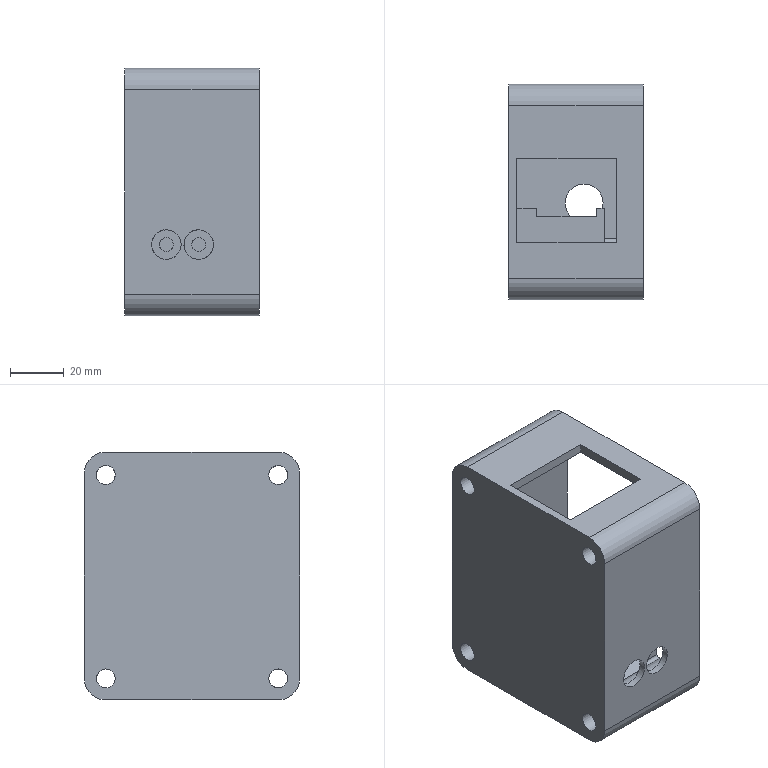NC program | NX | posted by the shop | part box 50 x 80 x 92 mm
Lines 1 to 169 of 30419:
%
O1234(1)
(T=1 D63 face mill Z=-30.00 D=63.00 R=0.00 L=30.00)
()
(T=3 Drill D7.0-73-105 Z=-73.00 D=7.00 R=0.00 L=105.00)
(T=4 Drill D4.0-54-83 Z=-54.00 D=4.00 R=0.00 L=83.00)
(T=5 D4-12-D4-50-3T-rough Z=-12.00 D=4.00 R=0.00 L=50.00)
(T=6 D12-36-D12-120-3T-finish Z=-45.00 D=12.00 R=0.00 L=120.00)
(T=7 D6-18-D6-50-3T-rough Z=-18.00 D=6.00 R=0.00 L=50.00)
(T=9 D2-6-D4-50-3T-rough Z=-6.00 D=2.00 R=0.00 L=7.00)
(T=10 D10-1 Z=-4.00 D=16.00 R=0.00 L=50.00)
()
(T=13 Drill D2.5-35-61 Z=-36.00 D=2.50 R=0.00 L=61.00)
(T=14 Spiral flute tap M3-10-D4-52 Z=-10.00 D=3.00 R=0.00 L=12.00)
G40 G17 G80 G90 G21
M9
M5
G91 G28 Z0.0
M1
N1
(T=1 N=D63 face mill D=1.00 R=0.00 FL=10.00 L=11.00)
(XY-STOCK=0.05)
T1 M6
T2
G0 G90 G54 X-22.5 Y-113. S4000 M3
G43 H01 Z30.
M8
Z3.
G1 Z0.0 F1000.
Y-50.
Y50.
Y113.
Z3.
G0 Z30.
X32.5 Y-113.
Z3.
G1 Z0.0
Y-50.
Y50.
Y113.
Z3.
G0 Z30.
M9
M5
G91 G28 Z0.0
M1
N2
(T=2 N=点孔D8-120-90度 D=8.00 R=0.00 FL=0.00 L=120.00)
(XY-STOCK=0.00)
T2 M6
T3
G0 G90 G54 X-40.5 Y17. S3000 M3
G43 H02 Z30.
M8
G98 G81 X-40.5 Y17. Z-1.5 R3. F200.
X-35.917 Y20.
X-29.422 Y27.
X-28.668 Y35.5
X-5.083 Y20.
X4.083
X29.168 Y35.5
X29.922 Y27.
X34.917 Y20.
X39.5 Y17.
Y-17.
X34.764 Y-20.027
X29.168 Y-35.5
X4.083 Y-20.
X-5.083
X-28.668 Y-35.5
X-29.422 Y-27.
X-35.917 Y-20.
G80
G0 X-35.917 Y-20. Z30.
G0 X-37.5 Y-32. S3000 M3
M8
G98 G81 X-37.5 Y-32. Z-1.5 R3. F200.
Y32.
X38.
Y-32.
G80
G0 X38. Y-32. Z30.
M9
M5
G91 G28 Z0.0
M1
N3
(T=3 N=Drill D7.0-73-105 D=7.00 R=0.00 FL=73.00 L=105.00)
(XY-STOCK=0.00)
T3 M6
T4
G0 G90 G54 X-37.5 Y-32. S3000 M3
G43 H03 Z30.
M8
G98 G83 X-37.5 Y-32. Z-54. R3. F250. Q2.
Y32.
X38.
Y-32.
G80
G0 X38. Y-32. Z30.
M9
M5
G91 G28 Z0.0
M1
N4
(T=4 N=Drill D4.0-54-83 D=4.00 R=0.00 FL=54.00 L=83.00)
(XY-STOCK=0.00)
T4 M6
T5
G0 G90 G54 X-40.5 Y17. S3000 M3
G43 H04 Z30.
M8
G98 G83 X-40.5 Y17. Z-47. R3. F200. Q2.
X-35.917 Y20.
X-29.422 Y27.
X-28.668 Y35.5
X-5.083 Y20.
X4.083
X29.168 Y35.5
X29.922 Y27.
X34.917 Y20.
X39.5 Y17.
Y-17.
X34.764 Y-20.027
X29.168 Y-35.5
X4.083 Y-20.
X-5.083
X-28.668 Y-35.5
X-29.422 Y-27.
X-35.917 Y-20.
G80
G0 X-35.917 Y-20. Z30.
M9
M5
G91 G28 Z0.0
M1
N5
(T=5 N=D4-12-D4-50-3T-rough D=4.00 R=0.00 FL=12.00 L=50.00)
(XY-STOCK=0.00)
T5 M6
T6
G0 G90 G54 X-40.5 Y17. S2000 M3
G43 H05 Z30.
M8
G98 G83 X-40.5 Y17. Z-47. R3. F150. Q2.
X-35.917 Y20.
X-29.422 Y27.
X-28.668 Y35.5
X-5.083 Y20.
X4.083
X29.168 Y35.5
X29.922 Y27.
X34.917 Y20.
X39.5 Y17.
Y-17.
X34.764 Y-20.027
X29.168 Y-35.5
X4.083 Y-20.
X-5.083
X-28.668 Y-35.5
X-29.422 Y-27.
X-35.917 Y-20.
G80
G0 X-35.917 Y-20. Z30.
M9
M5
G91 G28 Z0.0
M1
N6